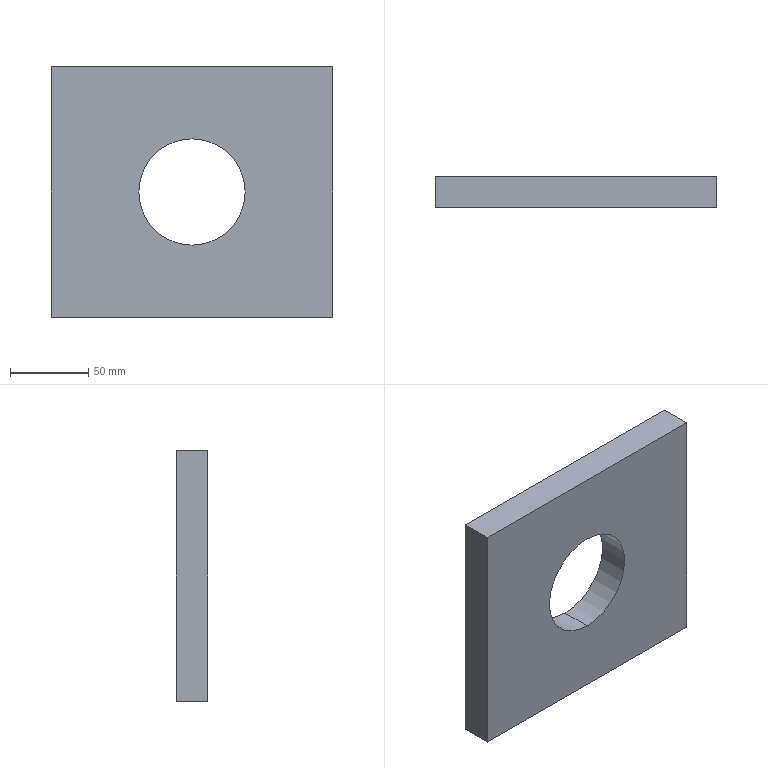Part | STEP file | Part10_5 | 1 solid | 8 faces | box 180 x 20 x 160 mm | volume 503407 mm3 | plane 6 | cylinder 2 | commonest cylinder face diameters 67.981 x2
STEP:
#1=CARTESIAN_POINT('',(0.,0.,0.));
#2=DIRECTION('',(0.,0.,1.));
#3=DIRECTION('',(1.,0.,0.));
#4=AXIS2_PLACEMENT_3D('',#1,#2,#3);
#5=CARTESIAN_POINT('',(90.7,-29.9,693.299));
#6=VERTEX_POINT('',#5);
#7=CARTESIAN_POINT('',(90.7,-9.9,693.299));
#8=VERTEX_POINT('',#7);
#9=CARTESIAN_POINT('',(90.7,-19.9,693.299));
#10=DIRECTION('',(0.,1.,0.));
#11=VECTOR('',#10,1.);
#12=LINE('',#9,#11);
#13=CARTESIAN_POINT('',(90.7,-19.9,659.308));
#14=DIRECTION('',(0.,1.,0.));
#15=DIRECTION('',(0.,0.,1.));
#16=AXIS2_PLACEMENT_3D('',#13,#14,#15);
#17=CYLINDRICAL_SURFACE('',#16,33.991);
#18=CARTESIAN_POINT('',(6.283,0.));
#19=DIRECTION('',(0.,1.));
#20=VECTOR('',#19,1.);
#21=LINE('',#18,#20);
#22=(GEOMETRIC_REPRESENTATION_CONTEXT(2)PARAMETRIC_REPRESENTATION_CONTEXT()REPRESENTATION_CONTEXT('',''));
#23=DEFINITIONAL_REPRESENTATION('',(#21),#22);
#24=PCURVE('',#17,#23);
#25=CARTESIAN_POINT('',(90.7,-19.9,659.308));
#26=DIRECTION('',(0.,1.,0.));
#27=DIRECTION('',(0.,0.,1.));
#28=AXIS2_PLACEMENT_3D('',#25,#26,#27);
#29=CYLINDRICAL_SURFACE('',#28,33.991);
#30=CARTESIAN_POINT('',(0.,0.));
#31=DIRECTION('',(0.,1.));
#32=VECTOR('',#31,1.);
#33=LINE('',#30,#32);
#34=(GEOMETRIC_REPRESENTATION_CONTEXT(2)PARAMETRIC_REPRESENTATION_CONTEXT()REPRESENTATION_CONTEXT('',''));
#35=DEFINITIONAL_REPRESENTATION('',(#33),#34);
#36=PCURVE('',#29,#35);
#37=SURFACE_CURVE('',#12,(#24,#36),.PCURVE_S1.);
#38=EDGE_CURVE('',#6,#8,#37,.T.);
#39=ORIENTED_EDGE('',*,*,#38,.T.);
#40=CARTESIAN_POINT('',(90.7,-9.9,625.318));
#41=VERTEX_POINT('',#40);
#42=CARTESIAN_POINT('',(90.7,-9.9,659.308));
#43=DIRECTION('',(0.,-1.,0.));
#44=DIRECTION('',(0.,0.,1.));
#45=AXIS2_PLACEMENT_3D('',#42,#43,#44);
#46=CIRCLE('',#45,33.991);
#47=CARTESIAN_POINT('',(6.283,10.));
#48=DIRECTION('',(-1.,0.));
#49=VECTOR('',#48,1.);
#50=LINE('',#47,#49);
#51=(GEOMETRIC_REPRESENTATION_CONTEXT(2)PARAMETRIC_REPRESENTATION_CONTEXT()REPRESENTATION_CONTEXT('',''));
#52=DEFINITIONAL_REPRESENTATION('',(#50),#51);
#53=PCURVE('',#17,#52);
#54=CARTESIAN_POINT('',(0.,-9.9,0.));
#55=DIRECTION('',(0.,1.,0.));
#56=DIRECTION('',(0.,0.,1.));
#57=AXIS2_PLACEMENT_3D('',#54,#55,#56);
#58=PLANE('',#57);
#59=CARTESIAN_POINT('',(693.299,90.7));
#60=CARTESIAN_POINT('',(693.299,31.827));
#61=CARTESIAN_POINT('',(642.313,61.264));
#62=CARTESIAN_POINT('',(591.327,90.7));
#63=CARTESIAN_POINT('',(642.313,120.137));
#64=CARTESIAN_POINT('',(693.299,149.574));
#65=CARTESIAN_POINT('',(693.299,90.7));
#66=(BOUNDED_CURVE()B_SPLINE_CURVE(2,(#59,#60,#61,#62,#63,#64,#65),.UNSPECIFIED.,.T.,.F.)B_SPLINE_CURVE_WITH_KNOTS((1,2,2,2,2,1),(-2.094,0.,2.094,4.189,6.283,8.378),.UNSPECIFIED.)CURVE()GEOMETRIC_REPRESENTATION_ITEM()RATIONAL_B_SPLINE_CURVE((1.,0.5,1.,0.5,1.,0.5,1.))REPRESENTATION_ITEM(''));
#67=(GEOMETRIC_REPRESENTATION_CONTEXT(2)PARAMETRIC_REPRESENTATION_CONTEXT()REPRESENTATION_CONTEXT('',''));
#68=DEFINITIONAL_REPRESENTATION('',(#66),#67);
#69=PCURVE('',#58,#68);
#70=SURFACE_CURVE('',#46,(#53,#69),.PCURVE_S1.);
#71=EDGE_CURVE('',#8,#41,#70,.T.);
#72=ORIENTED_EDGE('',*,*,#71,.T.);
#73=CARTESIAN_POINT('',(90.7,-29.9,625.318));
#74=VERTEX_POINT('',#73);
#75=CARTESIAN_POINT('',(90.7,-19.9,625.318));
#76=DIRECTION('',(0.,1.,0.));
#77=VECTOR('',#76,1.);
#78=LINE('',#75,#77);
#79=CARTESIAN_POINT('',(3.142,0.));
#80=DIRECTION('',(0.,1.));
#81=VECTOR('',#80,1.);
#82=LINE('',#79,#81);
#83=(GEOMETRIC_REPRESENTATION_CONTEXT(2)PARAMETRIC_REPRESENTATION_CONTEXT()REPRESENTATION_CONTEXT('',''));
#84=DEFINITIONAL_REPRESENTATION('',(#82),#83);
#85=PCURVE('',#17,#84);
#86=CARTESIAN_POINT('',(3.142,0.));
#87=DIRECTION('',(0.,1.));
#88=VECTOR('',#87,1.);
#89=LINE('',#86,#88);
#90=(GEOMETRIC_REPRESENTATION_CONTEXT(2)PARAMETRIC_REPRESENTATION_CONTEXT()REPRESENTATION_CONTEXT('',''));
#91=DEFINITIONAL_REPRESENTATION('',(#89),#90);
#92=PCURVE('',#29,#91);
#93=SURFACE_CURVE('',#78,(#85,#92),.PCURVE_S1.);
#94=EDGE_CURVE('',#74,#41,#93,.T.);
#95=ORIENTED_EDGE('',*,*,#94,.F.);
#96=CARTESIAN_POINT('',(90.7,-29.9,659.308));
#97=DIRECTION('',(0.,-1.,0.));
#98=DIRECTION('',(0.,0.,1.));
#99=AXIS2_PLACEMENT_3D('',#96,#97,#98);
#100=CIRCLE('',#99,33.991);
#101=CARTESIAN_POINT('',(6.283,-10.));
#102=DIRECTION('',(-1.,0.));
#103=VECTOR('',#102,1.);
#104=LINE('',#101,#103);
#105=(GEOMETRIC_REPRESENTATION_CONTEXT(2)PARAMETRIC_REPRESENTATION_CONTEXT()REPRESENTATION_CONTEXT('',''));
#106=DEFINITIONAL_REPRESENTATION('',(#104),#105);
#107=PCURVE('',#17,#106);
#108=CARTESIAN_POINT('',(0.,-29.9,0.));
#109=DIRECTION('',(0.,1.,0.));
#110=DIRECTION('',(0.,0.,1.));
#111=AXIS2_PLACEMENT_3D('',#108,#109,#110);
#112=PLANE('',#111);
#113=CARTESIAN_POINT('',(693.299,90.7));
#114=CARTESIAN_POINT('',(693.299,31.827));
#115=CARTESIAN_POINT('',(642.313,61.264));
#116=CARTESIAN_POINT('',(591.327,90.7));
#117=CARTESIAN_POINT('',(642.313,120.137));
#118=CARTESIAN_POINT('',(693.299,149.574));
#119=CARTESIAN_POINT('',(693.299,90.7));
#120=(BOUNDED_CURVE()B_SPLINE_CURVE(2,(#113,#114,#115,#116,#117,#118,#119),.UNSPECIFIED.,.T.,.F.)B_SPLINE_CURVE_WITH_KNOTS((1,2,2,2,2,1),(-2.094,0.,2.094,4.189,6.283,8.378),.UNSPECIFIED.)CURVE()GEOMETRIC_REPRESENTATION_ITEM()RATIONAL_B_SPLINE_CURVE((1.,0.5,1.,0.5,1.,0.5,1.))REPRESENTATION_ITEM(''));
#121=(GEOMETRIC_REPRESENTATION_CONTEXT(2)PARAMETRIC_REPRESENTATION_CONTEXT()REPRESENTATION_CONTEXT('',''));
#122=DEFINITIONAL_REPRESENTATION('',(#120),#121);
#123=PCURVE('',#112,#122);
#124=SURFACE_CURVE('',#100,(#107,#123),.PCURVE_S1.);
#125=EDGE_CURVE('',#6,#74,#124,.T.);
#126=ORIENTED_EDGE('',*,*,#125,.F.);
#127=EDGE_LOOP('',(#39,#72,#95,#126));
#128=FACE_BOUND('',#127,.F.);
#129=ADVANCED_FACE('',(#128),#17,.F.);
#130=ORIENTED_EDGE('',*,*,#71,.T.);
#131=CARTESIAN_POINT('',(90.7,-9.9,659.308));
#132=DIRECTION('',(0.,-1.,0.));
#133=DIRECTION('',(0.,0.,1.));
#134=AXIS2_PLACEMENT_3D('',#131,#132,#133);
#135=CIRCLE('',#134,33.991);
#136=CARTESIAN_POINT('',(693.299,90.7));
#137=CARTESIAN_POINT('',(693.299,31.827));
#138=CARTESIAN_POINT('',(642.313,61.264));
#139=CARTESIAN_POINT('',(591.327,90.7));
#140=CARTESIAN_POINT('',(642.313,120.137));
#141=CARTESIAN_POINT('',(693.299,149.574));
#142=CARTESIAN_POINT('',(693.299,90.7));
#143=(BOUNDED_CURVE()B_SPLINE_CURVE(2,(#136,#137,#138,#139,#140,#141,#142),.UNSPECIFIED.,.T.,.F.)B_SPLINE_CURVE_WITH_KNOTS((1,2,2,2,2,1),(-2.094,0.,2.094,4.189,6.283,8.378),.UNSPECIFIED.)CURVE()GEOMETRIC_REPRESENTATION_ITEM()RATIONAL_B_SPLINE_CURVE((1.,0.5,1.,0.5,1.,0.5,1.))REPRESENTATION_ITEM(''));
#144=(GEOMETRIC_REPRESENTATION_CONTEXT(2)PARAMETRIC_REPRESENTATION_CONTEXT()REPRESENTATION_CONTEXT('',''));
#145=DEFINITIONAL_REPRESENTATION('',(#143),#144);
#146=PCURVE('',#58,#145);
#147=CARTESIAN_POINT('',(6.283,10.));
#148=DIRECTION('',(-1.,0.));
#149=VECTOR('',#148,1.);
#150=LINE('',#147,#149);
#151=(GEOMETRIC_REPRESENTATION_CONTEXT(2)PARAMETRIC_REPRESENTATION_CONTEXT()REPRESENTATION_CONTEXT('',''));
#152=DEFINITIONAL_REPRESENTATION('',(#150),#151);
#153=PCURVE('',#29,#152);
#154=SURFACE_CURVE('',#135,(#146,#153),.PCURVE_S1.);
#155=EDGE_CURVE('',#41,#8,#154,.T.);
#156=ORIENTED_EDGE('',*,*,#155,.T.);
#157=EDGE_LOOP('',(#130,#156));
#158=FACE_BOUND('',#157,.T.);
#159=CARTESIAN_POINT('',(0.7002,-9.9,579.308));
#160=VERTEX_POINT('',#159);
#161=CARTESIAN_POINT('',(0.7002,-9.9,739.308));
#162=VERTEX_POINT('',#161);
#163=CARTESIAN_POINT('',(0.7002,-9.9,739.308));
#164=DIRECTION('',(0.,0.,1.));
#165=VECTOR('',#164,1.);
#166=LINE('',#163,#165);
#167=CARTESIAN_POINT('',(739.308,0.7002));
#168=DIRECTION('',(1.,0.));
#169=VECTOR('',#168,1.);
#170=LINE('',#167,#169);
#171=(GEOMETRIC_REPRESENTATION_CONTEXT(2)PARAMETRIC_REPRESENTATION_CONTEXT()REPRESENTATION_CONTEXT('',''));
#172=DEFINITIONAL_REPRESENTATION('',(#170),#171);
#173=PCURVE('',#58,#172);
#174=CARTESIAN_POINT('',(0.7002,-29.9,739.308));
#175=DIRECTION('',(1.,0.,0.));
#176=DIRECTION('',(0.,0.,-1.));
#177=AXIS2_PLACEMENT_3D('',#174,#175,#176);
#178=PLANE('',#177);
#179=CARTESIAN_POINT('',(0.,20.));
#180=DIRECTION('',(-1.,0.));
#181=VECTOR('',#180,1.);
#182=LINE('',#179,#181);
#183=(GEOMETRIC_REPRESENTATION_CONTEXT(2)PARAMETRIC_REPRESENTATION_CONTEXT()REPRESENTATION_CONTEXT('',''));
#184=DEFINITIONAL_REPRESENTATION('',(#182),#183);
#185=PCURVE('',#178,#184);
#186=SURFACE_CURVE('',#166,(#173,#185),.PCURVE_S1.);
#187=EDGE_CURVE('',#160,#162,#186,.T.);
#188=ORIENTED_EDGE('',*,*,#187,.T.);
#189=CARTESIAN_POINT('',(180.7,-9.9,739.308));
#190=VERTEX_POINT('',#189);
#191=CARTESIAN_POINT('',(180.7,-9.9,739.308));
#192=DIRECTION('',(1.,0.,0.));
#193=VECTOR('',#192,1.);
#194=LINE('',#191,#193);
#195=CARTESIAN_POINT('',(739.308,180.7));
#196=DIRECTION('',(0.,1.));
#197=VECTOR('',#196,1.);
#198=LINE('',#195,#197);
#199=(GEOMETRIC_REPRESENTATION_CONTEXT(2)PARAMETRIC_REPRESENTATION_CONTEXT()REPRESENTATION_CONTEXT('',''));
#200=DEFINITIONAL_REPRESENTATION('',(#198),#199);
#201=PCURVE('',#58,#200);
#202=CARTESIAN_POINT('',(180.7,-29.9,739.308));
#203=DIRECTION('',(0.,0.,-1.));
#204=DIRECTION('',(-1.,0.,0.));
#205=AXIS2_PLACEMENT_3D('',#202,#203,#204);
#206=PLANE('',#205);
#207=CARTESIAN_POINT('',(0.,20.));
#208=DIRECTION('',(-1.,0.));
#209=VECTOR('',#208,1.);
#210=LINE('',#207,#209);
#211=(GEOMETRIC_REPRESENTATION_CONTEXT(2)PARAMETRIC_REPRESENTATION_CONTEXT()REPRESENTATION_CONTEXT('',''));
#212=DEFINITIONAL_REPRESENTATION('',(#210),#211);
#213=PCURVE('',#206,#212);
#214=SURFACE_CURVE('',#194,(#201,#213),.PCURVE_S1.);
#215=EDGE_CURVE('',#162,#190,#214,.T.);
#216=ORIENTED_EDGE('',*,*,#215,.T.);
#217=CARTESIAN_POINT('',(180.7,-9.9,579.308));
#218=VERTEX_POINT('',#217);
#219=CARTESIAN_POINT('',(180.7,-9.9,579.308));
#220=DIRECTION('',(0.,0.,-1.));
#221=VECTOR('',#220,1.);
#222=LINE('',#219,#221);
#223=CARTESIAN_POINT('',(579.308,180.7));
#224=DIRECTION('',(-1.,0.));
#225=VECTOR('',#224,1.);
#226=LINE('',#223,#225);
#227=(GEOMETRIC_REPRESENTATION_CONTEXT(2)PARAMETRIC_REPRESENTATION_CONTEXT()REPRESENTATION_CONTEXT('',''));
#228=DEFINITIONAL_REPRESENTATION('',(#226),#227);
#229=PCURVE('',#58,#228);
#230=CARTESIAN_POINT('',(180.7,-29.9,579.308));
#231=DIRECTION('',(-1.,0.,0.));
#232=DIRECTION('',(0.,0.,1.));
#233=AXIS2_PLACEMENT_3D('',#230,#231,#232);
#234=PLANE('',#233);
#235=CARTESIAN_POINT('',(0.,20.));
#236=DIRECTION('',(-1.,0.));
#237=VECTOR('',#236,1.);
#238=LINE('',#235,#237);
#239=(GEOMETRIC_REPRESENTATION_CONTEXT(2)PARAMETRIC_REPRESENTATION_CONTEXT()REPRESENTATION_CONTEXT('',''));
#240=DEFINITIONAL_REPRESENTATION('',(#238),#239);
#241=PCURVE('',#234,#240);
#242=SURFACE_CURVE('',#222,(#229,#241),.PCURVE_S1.);
#243=EDGE_CURVE('',#190,#218,#242,.T.);
#244=ORIENTED_EDGE('',*,*,#243,.T.);
#245=CARTESIAN_POINT('',(0.7002,-9.9,579.308));
#246=DIRECTION('',(-1.,0.,0.));
#247=VECTOR('',#246,1.);
#248=LINE('',#245,#247);
#249=CARTESIAN_POINT('',(579.308,0.7002));
#250=DIRECTION('',(0.,-1.));
#251=VECTOR('',#250,1.);
#252=LINE('',#249,#251);
#253=(GEOMETRIC_REPRESENTATION_CONTEXT(2)PARAMETRIC_REPRESENTATION_CONTEXT()REPRESENTATION_CONTEXT('',''));
#254=DEFINITIONAL_REPRESENTATION('',(#252),#253);
#255=PCURVE('',#58,#254);
#256=CARTESIAN_POINT('',(0.7002,-29.9,579.308));
#257=DIRECTION('',(0.,0.,1.));
#258=DIRECTION('',(1.,0.,0.));
#259=AXIS2_PLACEMENT_3D('',#256,#257,#258);
#260=PLANE('',#259);
#261=CARTESIAN_POINT('',(0.,20.));
#262=DIRECTION('',(-1.,0.));
#263=VECTOR('',#262,1.);
#264=LINE('',#261,#263);
#265=(GEOMETRIC_REPRESENTATION_CONTEXT(2)PARAMETRIC_REPRESENTATION_CONTEXT()REPRESENTATION_CONTEXT('',''));
#266=DEFINITIONAL_REPRESENTATION('',(#264),#265);
#267=PCURVE('',#260,#266);
#268=SURFACE_CURVE('',#248,(#255,#267),.PCURVE_S1.);
#269=EDGE_CURVE('',#218,#160,#268,.T.);
#270=ORIENTED_EDGE('',*,*,#269,.T.);
#271=EDGE_LOOP('',(#188,#216,#244,#270));
#272=FACE_BOUND('',#271,.T.);
#273=ADVANCED_FACE('',(#158,#272),#58,.T.);
#274=CARTESIAN_POINT('',(180.7,-29.9,739.308));
#275=VERTEX_POINT('',#274);
#276=CARTESIAN_POINT('',(180.7,-29.9,579.308));
#277=VERTEX_POINT('',#276);
#278=CARTESIAN_POINT('',(180.7,-29.9,0.));
#279=DIRECTION('',(0.,0.,-1.));
#280=VECTOR('',#279,1.);
#281=LINE('',#278,#280);
#282=CARTESIAN_POINT('',(-579.308,0.));
#283=DIRECTION('',(-1.,0.));
#284=VECTOR('',#283,1.);
#285=LINE('',#282,#284);
#286=(GEOMETRIC_REPRESENTATION_CONTEXT(2)PARAMETRIC_REPRESENTATION_CONTEXT()REPRESENTATION_CONTEXT('',''));
#287=DEFINITIONAL_REPRESENTATION('',(#285),#286);
#288=PCURVE('',#234,#287);
#289=CARTESIAN_POINT('',(0.,180.7));
#290=DIRECTION('',(-1.,0.));
#291=VECTOR('',#290,1.);
#292=LINE('',#289,#291);
#293=(GEOMETRIC_REPRESENTATION_CONTEXT(2)PARAMETRIC_REPRESENTATION_CONTEXT()REPRESENTATION_CONTEXT('',''));
#294=DEFINITIONAL_REPRESENTATION('',(#292),#293);
#295=PCURVE('',#112,#294);
#296=SURFACE_CURVE('',#281,(#288,#295),.PCURVE_S1.);
#297=EDGE_CURVE('',#275,#277,#296,.T.);
#298=ORIENTED_EDGE('',*,*,#297,.T.);
#299=CARTESIAN_POINT('',(180.7,-29.9,579.308));
#300=DIRECTION('',(0.,1.,0.));
#301=VECTOR('',#300,1.);
#302=LINE('',#299,#301);
#303=CARTESIAN_POINT('',(0.,0.));
#304=DIRECTION('',(0.,1.));
#305=VECTOR('',#304,1.);
#306=LINE('',#303,#305);
#307=(GEOMETRIC_REPRESENTATION_CONTEXT(2)PARAMETRIC_REPRESENTATION_CONTEXT()REPRESENTATION_CONTEXT('',''));
#308=DEFINITIONAL_REPRESENTATION('',(#306),#307);
#309=PCURVE('',#234,#308);
#310=CARTESIAN_POINT('',(180.,0.));
#311=DIRECTION('',(0.,1.));
#312=VECTOR('',#311,1.);
#313=LINE('',#310,#312);
#314=(GEOMETRIC_REPRESENTATION_CONTEXT(2)PARAMETRIC_REPRESENTATION_CONTEXT()REPRESENTATION_CONTEXT('',''));
#315=DEFINITIONAL_REPRESENTATION('',(#313),#314);
#316=PCURVE('',#260,#315);
#317=SURFACE_CURVE('',#302,(#309,#316),.PCURVE_S1.);
#318=EDGE_CURVE('',#277,#218,#317,.T.);
#319=ORIENTED_EDGE('',*,*,#318,.T.);
#320=ORIENTED_EDGE('',*,*,#243,.F.);
#321=CARTESIAN_POINT('',(180.7,-29.9,739.308));
#322=DIRECTION('',(0.,-1.,0.));
#323=VECTOR('',#322,1.);
#324=LINE('',#321,#323);
#325=CARTESIAN_POINT('',(160.,0.));
#326=DIRECTION('',(0.,-1.));
#327=VECTOR('',#326,1.);
#328=LINE('',#325,#327);
#329=(GEOMETRIC_REPRESENTATION_CONTEXT(2)PARAMETRIC_REPRESENTATION_CONTEXT()REPRESENTATION_CONTEXT('',''));
#330=DEFINITIONAL_REPRESENTATION('',(#328),#329);
#331=PCURVE('',#234,#330);
#332=CARTESIAN_POINT('',(0.,0.));
#333=DIRECTION('',(0.,-1.));
#334=VECTOR('',#333,1.);
#335=LINE('',#332,#334);
#336=(GEOMETRIC_REPRESENTATION_CONTEXT(2)PARAMETRIC_REPRESENTATION_CONTEXT()REPRESENTATION_CONTEXT('',''));
#337=DEFINITIONAL_REPRESENTATION('',(#335),#336);
#338=PCURVE('',#206,#337);
#339=SURFACE_CURVE('',#324,(#331,#338),.PCURVE_S1.);
#340=EDGE_CURVE('',#190,#275,#339,.T.);
#341=ORIENTED_EDGE('',*,*,#340,.T.);
#342=EDGE_LOOP('',(#298,#319,#320,#341));
#343=FACE_BOUND('',#342,.T.);
#344=ADVANCED_FACE('',(#343),#234,.F.);
#345=CARTESIAN_POINT('',(0.7002,-29.9,579.308));
#346=VERTEX_POINT('',#345);
#347=CARTESIAN_POINT('',(0.,-29.9,579.308));
#348=DIRECTION('',(-1.,0.,0.));
#349=VECTOR('',#348,1.);
#350=LINE('',#347,#349);
#351=CARTESIAN_POINT('',(-0.7002,0.));
#352=DIRECTION('',(-1.,0.));
#353=VECTOR('',#352,1.);
#354=LINE('',#351,#353);
#355=(GEOMETRIC_REPRESENTATION_CONTEXT(2)PARAMETRIC_REPRESENTATION_CONTEXT()REPRESENTATION_CONTEXT('',''));
#356=DEFINITIONAL_REPRESENTATION('',(#354),#355);
#357=PCURVE('',#260,#356);
#358=CARTESIAN_POINT('',(579.308,0.));
#359=DIRECTION('',(0.,-1.));
#360=VECTOR('',#359,1.);
#361=LINE('',#358,#360);
#362=(GEOMETRIC_REPRESENTATION_CONTEXT(2)PARAMETRIC_REPRESENTATION_CONTEXT()REPRESENTATION_CONTEXT('',''));
#363=DEFINITIONAL_REPRESENTATION('',(#361),#362);
#364=PCURVE('',#112,#363);
#365=SURFACE_CURVE('',#350,(#357,#364),.PCURVE_S1.);
#366=EDGE_CURVE('',#277,#346,#365,.T.);
#367=ORIENTED_EDGE('',*,*,#366,.T.);
#368=CARTESIAN_POINT('',(0.7002,-29.9,579.308));
#369=DIRECTION('',(0.,1.,0.));
#370=VECTOR('',#369,1.);
#371=LINE('',#368,#370);
#372=CARTESIAN_POINT('',(0.,0.));
#373=DIRECTION('',(0.,1.));
#374=VECTOR('',#373,1.);
#375=LINE('',#372,#374);
#376=(GEOMETRIC_REPRESENTATION_CONTEXT(2)PARAMETRIC_REPRESENTATION_CONTEXT()REPRESENTATION_CONTEXT('',''));
#377=DEFINITIONAL_REPRESENTATION('',(#375),#376);
#378=PCURVE('',#260,#377);
#379=CARTESIAN_POINT('',(160.,0.));
#380=DIRECTION('',(0.,1.));
#381=VECTOR('',#380,1.);
#382=LINE('',#379,#381);
#383=(GEOMETRIC_REPRESENTATION_CONTEXT(2)PARAMETRIC_REPRESENTATION_CONTEXT()REPRESENTATION_CONTEXT('',''));
#384=DEFINITIONAL_REPRESENTATION('',(#382),#383);
#385=PCURVE('',#178,#384);
#386=SURFACE_CURVE('',#371,(#378,#385),.PCURVE_S1.);
#387=EDGE_CURVE('',#346,#160,#386,.T.);
#388=ORIENTED_EDGE('',*,*,#387,.T.);
#389=ORIENTED_EDGE('',*,*,#269,.F.);
#390=ORIENTED_EDGE('',*,*,#318,.F.);
#391=EDGE_LOOP('',(#367,#388,#389,#390));
#392=FACE_BOUND('',#391,.T.);
#393=ADVANCED_FACE('',(#392),#260,.F.);
#394=CARTESIAN_POINT('',(0.7002,-29.9,739.308));
#395=VERTEX_POINT('',#394);
#396=CARTESIAN_POINT('',(0.7002,-29.9,0.));
#397=DIRECTION('',(0.,0.,1.));
#398=VECTOR('',#397,1.);
#399=LINE('',#396,#398);
#400=CARTESIAN_POINT('',(739.308,0.));
#401=DIRECTION('',(-1.,0.));
#402=VECTOR('',#401,1.);
#403=LINE('',#400,#402);
#404=(GEOMETRIC_REPRESENTATION_CONTEXT(2)PARAMETRIC_REPRESENTATION_CONTEXT()REPRESENTATION_CONTEXT('',''));
#405=DEFINITIONAL_REPRESENTATION('',(#403),#404);
#406=PCURVE('',#178,#405);
#407=CARTESIAN_POINT('',(0.,0.7002));
#408=DIRECTION('',(1.,0.));
#409=VECTOR('',#408,1.);
#410=LINE('',#407,#409);
#411=(GEOMETRIC_REPRESENTATION_CONTEXT(2)PARAMETRIC_REPRESENTATION_CONTEXT()REPRESENTATION_CONTEXT('',''));
#412=DEFINITIONAL_REPRESENTATION('',(#410),#411);
#413=PCURVE('',#112,#412);
#414=SURFACE_CURVE('',#399,(#406,#413),.PCURVE_S1.);
#415=EDGE_CURVE('',#346,#395,#414,.T.);
#416=ORIENTED_EDGE('',*,*,#415,.T.);
#417=CARTESIAN_POINT('',(0.7002,-29.9,739.308));
#418=DIRECTION('',(0.,1.,0.));
#419=VECTOR('',#418,1.);
#420=LINE('',#417,#419);
#421=CARTESIAN_POINT('',(0.,0.));
#422=DIRECTION('',(0.,1.));
#423=VECTOR('',#422,1.);
#424=LINE('',#421,#423);
#425=(GEOMETRIC_REPRESENTATION_CONTEXT(2)PARAMETRIC_REPRESENTATION_CONTEXT()REPRESENTATION_CONTEXT('',''));
#426=DEFINITIONAL_REPRESENTATION('',(#424),#425);
#427=PCURVE('',#178,#426);
#428=CARTESIAN_POINT('',(180.,0.));
#429=DIRECTION('',(0.,1.));
#430=VECTOR('',#429,1.);
#431=LINE('',#428,#430);
#432=(GEOMETRIC_REPRESENTATION_CONTEXT(2)PARAMETRIC_REPRESENTATION_CONTEXT()REPRESENTATION_CONTEXT('',''));
#433=DEFINITIONAL_REPRESENTATION('',(#431),#432);
#434=PCURVE('',#206,#433);
#435=SURFACE_CURVE('',#420,(#427,#434),.PCURVE_S1.);
#436=EDGE_CURVE('',#395,#162,#435,.T.);
#437=ORIENTED_EDGE('',*,*,#436,.T.);
#438=ORIENTED_EDGE('',*,*,#187,.F.);
#439=ORIENTED_EDGE('',*,*,#387,.F.);
#440=EDGE_LOOP('',(#416,#437,#438,#439));
#441=FACE_BOUND('',#440,.T.);
#442=ADVANCED_FACE('',(#441),#178,.F.);
#443=CARTESIAN_POINT('',(0.,-29.9,739.308));
#444=DIRECTION('',(1.,0.,0.));
#445=VECTOR('',#444,1.);
#446=LINE('',#443,#445);
#447=CARTESIAN_POINT('',(180.7,0.));
#448=DIRECTION('',(-1.,0.));
#449=VECTOR('',#448,1.);
#450=LINE('',#447,#449);
#451=(GEOMETRIC_REPRESENTATION_CONTEXT(2)PARAMETRIC_REPRESENTATION_CONTEXT()REPRESENTATION_CONTEXT('',''));
#452=DEFINITIONAL_REPRESENTATION('',(#450),#451);
#453=PCURVE('',#206,#452);
#454=CARTESIAN_POINT('',(739.308,0.));
#455=DIRECTION('',(0.,1.));
#456=VECTOR('',#455,1.);
#457=LINE('',#454,#456);
#458=(GEOMETRIC_REPRESENTATION_CONTEXT(2)PARAMETRIC_REPRESENTATION_CONTEXT()REPRESENTATION_CONTEXT('',''));
#459=DEFINITIONAL_REPRESENTATION('',(#457),#458);
#460=PCURVE('',#112,#459);
#461=SURFACE_CURVE('',#446,(#453,#460),.PCURVE_S1.);
#462=EDGE_CURVE('',#395,#275,#461,.T.);
#463=ORIENTED_EDGE('',*,*,#462,.T.);
#464=ORIENTED_EDGE('',*,*,#340,.F.);
#465=ORIENTED_EDGE('',*,*,#215,.F.);
#466=ORIENTED_EDGE('',*,*,#436,.F.);
#467=EDGE_LOOP('',(#463,#464,#465,#466));
#468=FACE_BOUND('',#467,.T.);
#469=ADVANCED_FACE('',(#468),#206,.F.);
#470=ORIENTED_EDGE('',*,*,#155,.T.);
#471=ORIENTED_EDGE('',*,*,#38,.F.);
#472=CARTESIAN_POINT('',(90.7,-29.9,659.308));
#473=DIRECTION('',(0.,-1.,0.));
#474=DIRECTION('',(0.,0.,1.));
#475=AXIS2_PLACEMENT_3D('',#472,#473,#474);
#476=CIRCLE('',#475,33.991);
#477=CARTESIAN_POINT('',(6.283,-10.));
#478=DIRECTION('',(-1.,0.));
#479=VECTOR('',#478,1.);
#480=LINE('',#477,#479);
#481=(GEOMETRIC_REPRESENTATION_CONTEXT(2)PARAMETRIC_REPRESENTATION_CONTEXT()REPRESENTATION_CONTEXT('',''));
#482=DEFINITIONAL_REPRESENTATION('',(#480),#481);
#483=PCURVE('',#29,#482);
#484=CARTESIAN_POINT('',(693.299,90.7));
#485=CARTESIAN_POINT('',(693.299,31.827));
#486=CARTESIAN_POINT('',(642.313,61.264));
#487=CARTESIAN_POINT('',(591.327,90.7));
#488=CARTESIAN_POINT('',(642.313,120.137));
#489=CARTESIAN_POINT('',(693.299,149.574));
#490=CARTESIAN_POINT('',(693.299,90.7));
#491=(BOUNDED_CURVE()B_SPLINE_CURVE(2,(#484,#485,#486,#487,#488,#489,#490),.UNSPECIFIED.,.T.,.F.)B_SPLINE_CURVE_WITH_KNOTS((1,2,2,2,2,1),(-2.094,0.,2.094,4.189,6.283,8.378),.UNSPECIFIED.)CURVE()GEOMETRIC_REPRESENTATION_ITEM()RATIONAL_B_SPLINE_CURVE((1.,0.5,1.,0.5,1.,0.5,1.))REPRESENTATION_ITEM(''));
#492=(GEOMETRIC_REPRESENTATION_CONTEXT(2)PARAMETRIC_REPRESENTATION_CONTEXT()REPRESENTATION_CONTEXT('',''));
#493=DEFINITIONAL_REPRESENTATION('',(#491),#492);
#494=PCURVE('',#112,#493);
#495=SURFACE_CURVE('',#476,(#483,#494),.PCURVE_S1.);
#496=EDGE_CURVE('',#74,#6,#495,.T.);
#497=ORIENTED_EDGE('',*,*,#496,.F.);
#498=ORIENTED_EDGE('',*,*,#94,.T.);
#499=EDGE_LOOP('',(#470,#471,#497,#498));
#500=FACE_BOUND('',#499,.F.);
#501=ADVANCED_FACE('',(#500),#29,.F.);
#502=ORIENTED_EDGE('',*,*,#125,.F.);
#503=ORIENTED_EDGE('',*,*,#496,.F.);
#504=EDGE_LOOP('',(#502,#503));
#505=FACE_BOUND('',#504,.T.);
#506=ORIENTED_EDGE('',*,*,#415,.F.);
#507=ORIENTED_EDGE('',*,*,#366,.F.);
#508=ORIENTED_EDGE('',*,*,#297,.F.);
#509=ORIENTED_EDGE('',*,*,#462,.F.);
#510=EDGE_LOOP('',(#506,#507,#508,#509));
#511=FACE_BOUND('',#510,.T.);
#512=ADVANCED_FACE('',(#505,#511),#112,.F.);
#513=CLOSED_SHELL('',(#129,#273,#344,#393,#442,#469,#501,#512));
#514=MANIFOLD_SOLID_BREP('',#513);
#515=(LENGTH_UNIT()NAMED_UNIT(*)SI_UNIT(.MILLI.,.METRE.));
#516=UNCERTAINTY_MEASURE_WITH_UNIT(LENGTH_MEASURE(0.0000001),#515,'','');
#517=(NAMED_UNIT(*)PLANE_ANGLE_UNIT()SI_UNIT($,.RADIAN.));
#518=(NAMED_UNIT(*)SI_UNIT($,.STERADIAN.)SOLID_ANGLE_UNIT());
#519=(GEOMETRIC_REPRESENTATION_CONTEXT(3)GLOBAL_UNCERTAINTY_ASSIGNED_CONTEXT((#516))GLOBAL_UNIT_ASSIGNED_CONTEXT((#515,#517,#518))REPRESENTATION_CONTEXT('',''));
#520=ADVANCED_BREP_SHAPE_REPRESENTATION('',(#4,#514),#519);